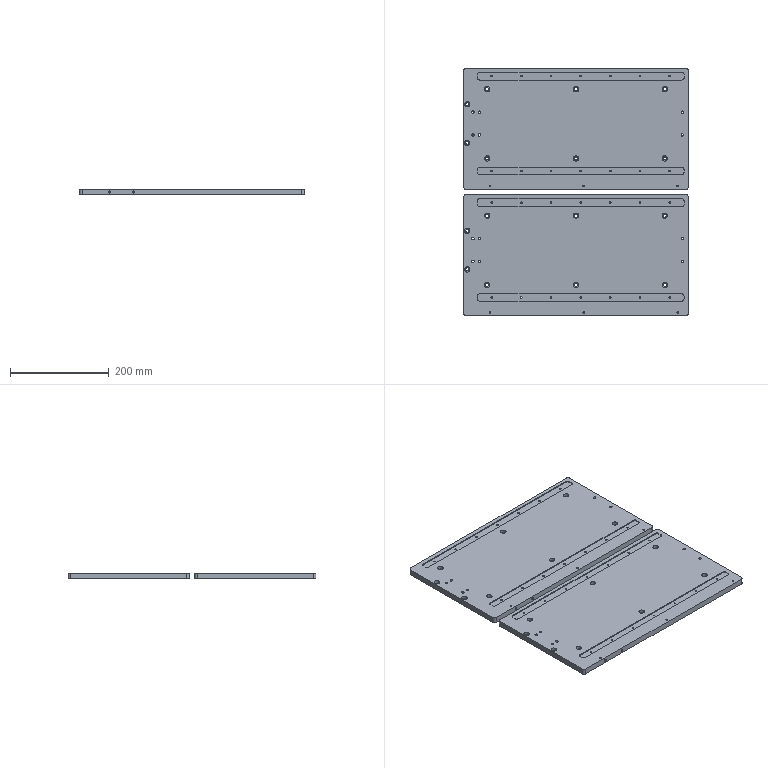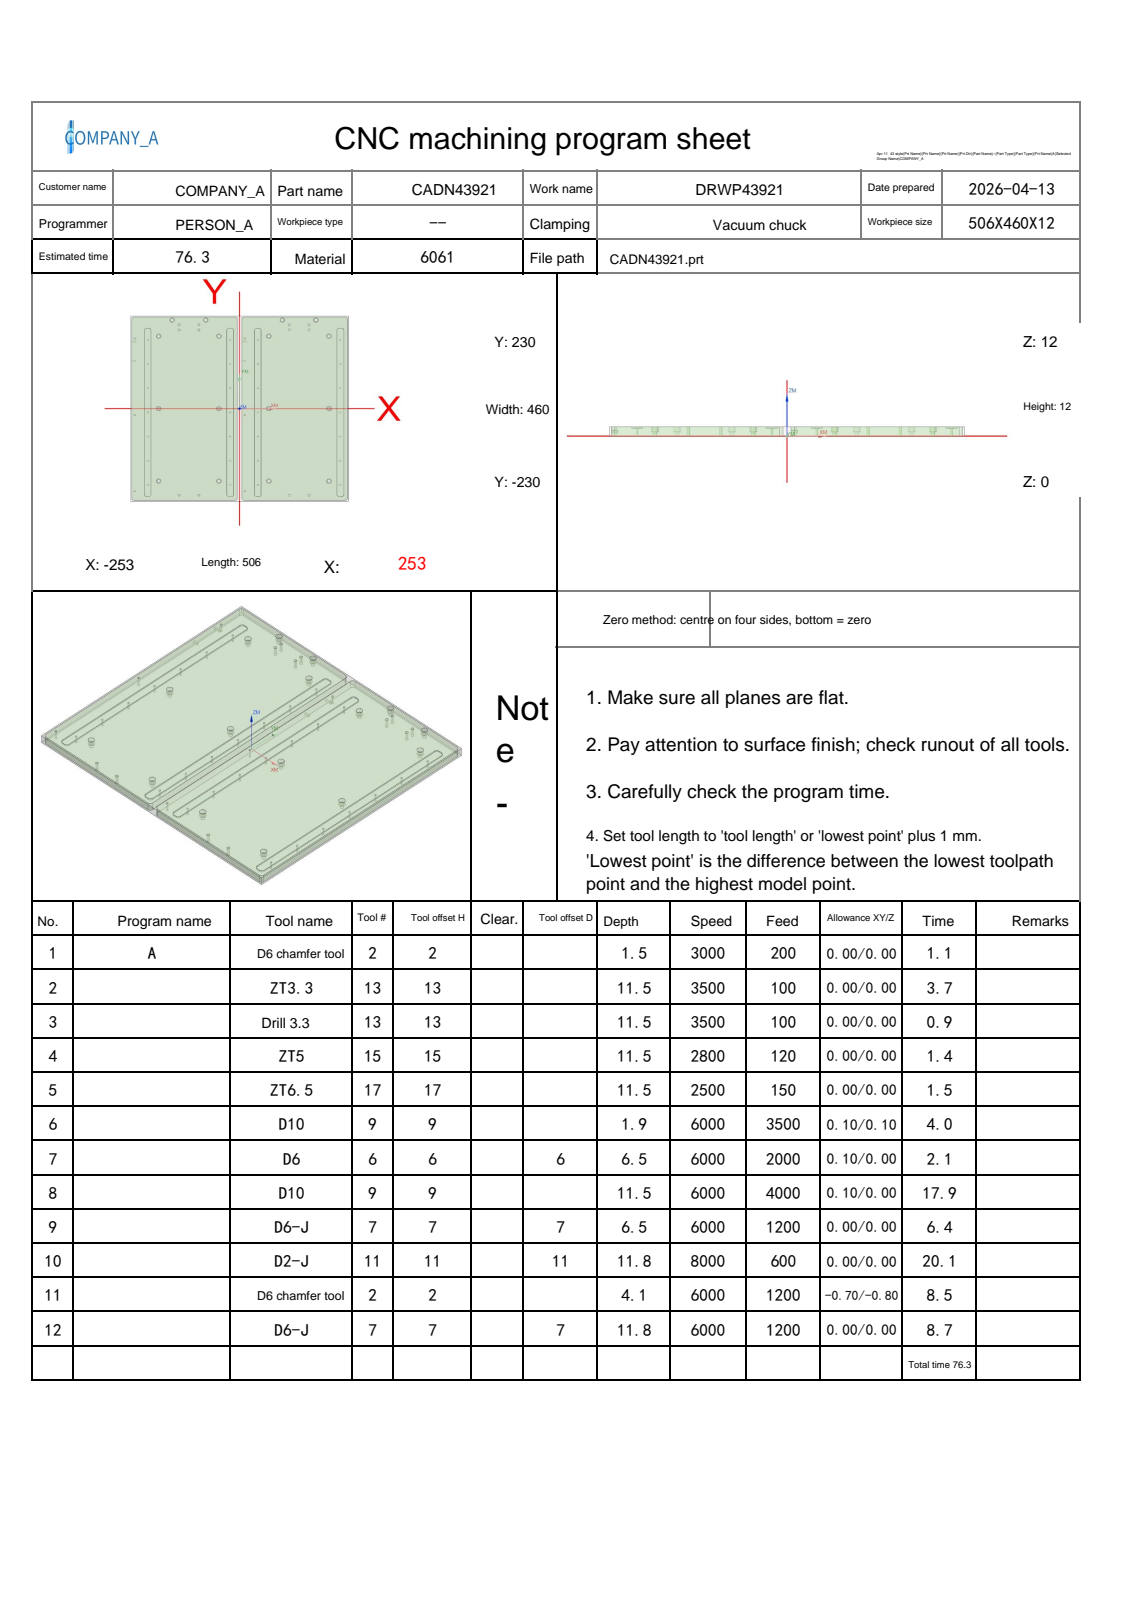NC program | NX | posted by the shop | part box 455 x 501 x 12 mm
Lines 10875 to 11580 of 11580:
N11 T02 M06
(D6 chamfer tool  D=6. R=0. H=02 ce=0.00 di=0.00)
G00 G90 G54 X3.672 Y-.25 M03 S6000
G43 H02 Z32.
M08
Z14.399
G01 Z10.501 F1200.
G03 X3.972 Y-.33 I.3 J.52
X4.492 Y-.03 I0.0 J.6
G01 X4.5 Y0.0
Y222.5
G02 X10.5 Y228.5 I6. J0.0
G01 X245.5
G02 X251.5 Y222.5 I0.0 J-6.
G01 Y-222.5
G02 X245.5 Y-228.5 I-6. J0.0
G01 X10.5
G02 X4.5 Y-222.5 I0.0 J6.
G01 Y0.0
X4.492 Y.03
G03 X3.972 Y.33 I-.52 J-.3
X3.672 Y.25 I0.0 J-.6
G01 Z14.399
G00 Z32.
X228.328 Y-9.25
Z14.399
G01 Z10.501
G03 X228.028 Y-9.17 I-.3 J-.52
X227.508 Y-9.47 I0.0 J-.6
G01 X227.5 Y-9.5
Y-213.5
G03 X231.7 Y-217.7 I4.2 J0.0
G01 X237.3
G03 X241.5 Y-213.5 I0.0 J4.2
G01 Y194.5
G03 X237.3 Y198.7 I-4.2 J0.0
G01 X231.7
G03 X227.5 Y194.5 I0.0 J-4.2
G01 Y-9.5
X227.508 Y-9.53
G03 X228.028 Y-9.83 I.52 J.3
X228.328 Y-9.75 I0.0 J.6
G01 Z14.399
G00 Z32.
X48.222
Z14.399
G01 Z10.501
G03 X48.522 Y-9.83 I.3 J.52
X49.042 Y-9.53 I0.0 J.6
G01 X49.05 Y-9.5
Y194.5
G03 X45. Y198.55 I-4.05 J0.0
G01 X40.
G03 X35.95 Y194.5 I0.0 J-4.05
G01 Y-213.5
G03 X40. Y-217.55 I4.05 J0.0
G01 X45.
G03 X49.05 Y-213.5 I0.0 J4.05
G01 Y-9.5
X49.042 Y-9.47
G03 X48.522 Y-9.17 I-.52 J-.3
X48.222 Y-9.25 I0.0 J-.6
G01 Z14.399
G00 Z32.
X-3.672 Y.25
Z14.399
G01 Z10.501
G03 X-3.972 Y.33 I-.3 J-.52
X-4.492 Y.03 I0.0 J-.6
G01 X-4.5 Y0.0
Y-222.5
G02 X-10.5 Y-228.5 I-6. J0.0
G01 X-245.5
G02 X-251.5 Y-222.5 I0.0 J6.
G01 Y222.5
G02 X-245.5 Y228.5 I6. J0.0
G01 X-10.5
G02 X-4.5 Y222.5 I0.0 J-6.
G01 Y0.0
X-4.492 Y-.03
G03 X-3.972 Y-.33 I.52 J.3
X-3.672 Y-.25 I0.0 J.6
G01 Z14.399
G00 Z32.
X-15.328 Y-9.75
Z14.399
G01 Z10.501
G03 X-15.028 Y-9.83 I.3 J.52
X-14.508 Y-9.53 I0.0 J.6
G01 X-14.5 Y-9.5
Y194.5
G03 X-18.7 Y198.7 I-4.2 J0.0
G01 X-24.3
G03 X-28.5 Y194.5 I0.0 J-4.2
G01 Y-213.5
G03 X-24.3 Y-217.7 I4.2 J0.0
G01 X-18.7
G03 X-14.5 Y-213.5 I0.0 J4.2
G01 Y-9.5
X-14.508 Y-9.47
G03 X-15.028 Y-9.17 I-.52 J-.3
X-15.328 Y-9.25 I0.0 J-.6
G01 Z14.399
G00 Z32.
X-207.778 Y-9.75
Z14.399
G01 Z10.501
G03 X-207.478 Y-9.83 I.3 J.52
X-206.958 Y-9.53 I0.0 J.6
G01 X-206.95 Y-9.5
Y194.5
G03 X-211. Y198.55 I-4.05 J0.0
G01 X-216.
G03 X-220.05 Y194.5 I0.0 J-4.05
G01 Y-213.5
G03 X-216. Y-217.55 I4.05 J0.0
G01 X-211.
G03 X-206.95 Y-213.5 I0.0 J4.05
G01 Y-9.5
X-206.958 Y-9.47
G03 X-207.478 Y-9.17 I-.52 J-.3
X-207.778 Y-9.25 I0.0 J-.6
G01 Z14.399
G00 Z32.
G00 G90 X-213.5 Y-189.5 M03 S5000
Z32.
G98 G81 X-213.5 Y-189.5 Z7.85 R13. F150.
Y-129.5
Y-69.5
Y-9.5
Y50.5
Y110.5
Y170.5
X-21.5 Y110.5
Y170.5
X42.5
Y110.5
Y50.5
X-21.5
Y-9.5
X42.5
Y-69.5
X-21.5
Y-129.5
Y-189.5
X42.5
Y-129.5
X234.5 Y-189.5
Y-129.5
Y-69.5
Y-9.5
Y50.5
Y110.5
Y170.5
G80
G00 Z32.
G00 G90 X-244. Y-205.678 M03 S5000
Z32.
G98 G81 X-244. Y-205.678 Z9.8 R15. F150.
Y-15.678
Y174.322
X12.
Y-15.678
Y-205.678
G80
G00 Z32.
G00 G90 X162.099 Y195.54 M03 S6000
Z32.
Z10.9
G01 Z10.4 F600.
X163. Y195.6
G03 X161.5 Y197.1 I-1.5 J0.0
X159.9 Y195.5 I0.0 J-1.6
X161.5 Y193.9 I1.6 J0.0
X163.1 Y195.5 I0.0 J1.6
X161.5 Y197.1 I-1.6 J0.0
X160. Y195.6 I0.0 J-1.5
G01 X160.901 Y195.54
Z10.9
G00 Z32.
X162.099 Y208.54
Z10.9
G01 Z10.4
X163. Y208.6
G03 X161.5 Y210.1 I-1.5 J0.0
X159.9 Y208.5 I0.0 J-1.6
X161.5 Y206.9 I1.6 J0.0
X163.1 Y208.5 I0.0 J1.6
X161.5 Y210.1 I-1.6 J0.0
X160. Y208.6 I0.0 J-1.5
G01 X160.901 Y208.54
Z10.9
G00 Z32.
X116.099
Z10.9
G01 Z10.4
X117. Y208.6
G03 X115.5 Y210.1 I-1.5 J0.0
X113.9 Y208.5 I0.0 J-1.6
X115.5 Y206.9 I1.6 J0.0
X117.1 Y208.5 I0.0 J1.6
X115.5 Y210.1 I-1.6 J0.0
X114. Y208.6 I0.0 J-1.5
G01 X114.901 Y208.54
Z10.9
G00 Z32.
X116.099 Y195.54
Z10.9
G01 Z10.4
X117. Y195.6
G03 X115.5 Y197.1 I-1.5 J0.0
X113.9 Y195.5 I0.0 J-1.6
X115.5 Y193.9 I1.6 J0.0
X117.1 Y195.5 I0.0 J1.6
X115.5 Y197.1 I-1.6 J0.0
X114. Y195.6 I0.0 J-1.5
G01 X114.901 Y195.54
Z10.9
G00 Z32.
X-93.901
Z10.9
G01 Z10.4
X-93. Y195.6
G03 X-94.5 Y197.1 I-1.5 J0.0
X-96.1 Y195.5 I0.0 J-1.6
X-94.5 Y193.9 I1.6 J0.0
X-92.9 Y195.5 I0.0 J1.6
X-94.5 Y197.1 I-1.6 J0.0
X-96. Y195.6 I0.0 J-1.5
G01 X-95.099 Y195.54
Z10.9
G00 Z32.
X-93.901 Y208.54
Z10.9
G01 Z10.4
X-93. Y208.6
G03 X-94.5 Y210.1 I-1.5 J0.0
X-96.1 Y208.5 I0.0 J-1.6
X-94.5 Y206.9 I1.6 J0.0
X-92.9 Y208.5 I0.0 J1.6
X-94.5 Y210.1 I-1.6 J0.0
X-96. Y208.6 I0.0 J-1.5
G01 X-95.099 Y208.54
Z10.9
G00 Z32.
X-139.901
Z10.9
G01 Z10.4
X-139. Y208.6
G03 X-140.5 Y210.1 I-1.5 J0.0
X-142.1 Y208.5 I0.0 J-1.6
X-140.5 Y206.9 I1.6 J0.0
X-138.9 Y208.5 I0.0 J1.6
X-140.5 Y210.1 I-1.6 J0.0
X-142. Y208.6 I0.0 J-1.5
G01 X-141.099 Y208.54
Z10.9
G00 Z32.
X-139.901 Y195.54
Z10.9
G01 Z10.4
X-139. Y195.6
G03 X-140.5 Y197.1 I-1.5 J0.0
X-142.1 Y195.5 I0.0 J-1.6
X-140.5 Y193.9 I1.6 J0.0
X-138.9 Y195.5 I0.0 J1.6
X-140.5 Y197.1 I-1.6 J0.0
X-142. Y195.6 I0.0 J-1.5
G01 X-141.099 Y195.54
Z10.9
G00 Z32.
X-139.901 Y-214.96
Z10.9
G01 Z10.4
X-139. Y-214.9
G03 X-140.5 Y-213.4 I-1.5 J0.0
X-142.1 Y-215. I0.0 J-1.6
X-140.5 Y-216.6 I1.6 J0.0
X-138.9 Y-215. I0.0 J1.6
X-140.5 Y-213.4 I-1.6 J0.0
X-142. Y-214.9 I0.0 J-1.5
G01 X-141.099 Y-214.96
Z10.9
G00 Z32.
X-93.901
Z10.9
G01 Z10.4
X-93. Y-214.9
G03 X-94.5 Y-213.4 I-1.5 J0.0
X-96.1 Y-215. I0.0 J-1.6
X-94.5 Y-216.6 I1.6 J0.0
X-92.9 Y-215. I0.0 J1.6
X-94.5 Y-213.4 I-1.6 J0.0
X-96. Y-214.9 I0.0 J-1.5
G01 X-95.099 Y-214.96
Z10.9
G00 Z32.
X116.099
Z10.9
G01 Z10.4
X117. Y-214.9
G03 X115.5 Y-213.4 I-1.5 J0.0
X113.9 Y-215. I0.0 J-1.6
X115.5 Y-216.6 I1.6 J0.0
X117.1 Y-215. I0.0 J1.6
X115.5 Y-213.4 I-1.6 J0.0
X114. Y-214.9 I0.0 J-1.5
G01 X114.901 Y-214.96
Z10.9
G00 Z32.
X162.099
Z10.9
G01 Z10.4
X163. Y-214.9
G03 X161.5 Y-213.4 I-1.5 J0.0
X159.9 Y-215. I0.0 J-1.6
X161.5 Y-216.6 I1.6 J0.0
X163.1 Y-215. I0.0 J1.6
X161.5 Y-213.4 I-1.6 J0.0
X160. Y-214.9 I0.0 J-1.5
G01 X160.901 Y-214.96
Z10.9
G00 Z32.
G00 G90 X211. Y180.001 M03 S6000
Z32.
Z10.5
G01 Z10. F600.
Y181.
G03 X208. Y184. I-3. J0.0
X204. Y180. I0.0 J-4.
X208. Y176. I4. J0.0
X212. Y180. I0.0 J4.
X208. Y184. I-4. J0.0
X205. Y181. I0.0 J-3.
G01 Y180.001
Z10.5
G00 Z32.
X180.5 Y220.001
Z10.5
G01 Z10.
Y221.
G03 X177.5 Y224. I-3. J0.0
X173.5 Y220. I0.0 J-4.
X177.5 Y216. I4. J0.0
X181.5 Y220. I0.0 J4.
X177.5 Y224. I-4. J0.0
X174.5 Y221. I0.0 J-3.
G01 Y220.001
Z10.5
G00 Z32.
X102.5
Z10.5
G01 Z10.
Y221.
G03 X99.5 Y224. I-3. J0.0
X95.5 Y220. I0.0 J-4.
X99.5 Y216. I4. J0.0
X103.5 Y220. I0.0 J4.
X99.5 Y224. I-4. J0.0
X96.5 Y221. I0.0 J-3.
G01 Y220.001
Z10.5
G00 Z32.
X71. Y180.001
Z10.5
G01 Z10.
Y181.
G03 X68. Y184. I-3. J0.0
X64. Y180. I0.0 J-4.
X68. Y176. I4. J0.0
X72. Y180. I0.0 J4.
X68. Y184. I-4. J0.0
X65. Y181. I0.0 J-3.
G01 Y180.001
Z10.5
G00 Z32.
X-45.
Z10.5
G01 Z10.
Y181.
G03 X-48. Y184. I-3. J0.0
X-52. Y180. I0.0 J-4.
X-48. Y176. I4. J0.0
X-44. Y180. I0.0 J4.
X-48. Y184. I-4. J0.0
X-51. Y181. I0.0 J-3.
G01 Y180.001
Z10.5
G00 Z32.
X-75.5 Y220.001
Z10.5
G01 Z10.
Y221.
G03 X-78.5 Y224. I-3. J0.0
X-82.5 Y220. I0.0 J-4.
X-78.5 Y216. I4. J0.0
X-74.5 Y220. I0.0 J4.
X-78.5 Y224. I-4. J0.0
X-81.5 Y221. I0.0 J-3.
G01 Y220.001
Z10.5
G00 Z32.
X-153.5
Z10.5
G01 Z10.
Y221.
G03 X-156.5 Y224. I-3. J0.0
X-160.5 Y220. I0.0 J-4.
X-156.5 Y216. I4. J0.0
X-152.5 Y220. I0.0 J4.
X-156.5 Y224. I-4. J0.0
X-159.5 Y221. I0.0 J-3.
G01 Y220.001
Z10.5
G00 Z32.
X-185. Y180.001
Z10.5
G01 Z10.
Y181.
G03 X-188. Y184. I-3. J0.0
X-192. Y180. I0.0 J-4.
X-188. Y176. I4. J0.0
X-184. Y180. I0.0 J4.
X-188. Y184. I-4. J0.0
X-191. Y181. I0.0 J-3.
G01 Y180.001
Z10.5
G00 Z32.
X-185. Y.001
Z10.5
G01 Z10.
Y1.
G03 X-188. Y4. I-3. J0.0
X-192. Y0.0 I0.0 J-4.
X-188. Y-4. I4. J0.0
X-184. Y0.0 I0.0 J4.
X-188. Y4. I-4. J0.0
X-191. Y1. I0.0 J-3.
G01 Y.001
Z10.5
G00 Z32.
X-45.
Z10.5
G01 Z10.
Y1.
G03 X-48. Y4. I-3. J0.0
X-52. Y0.0 I0.0 J-4.
X-48. Y-4. I4. J0.0
X-44. Y0.0 I0.0 J4.
X-48. Y4. I-4. J0.0
X-51. Y1. I0.0 J-3.
G01 Y.001
Z10.5
G00 Z32.
X71.
Z10.5
G01 Z10.
Y1.
G03 X68. Y4. I-3. J0.0
X64. Y0.0 I0.0 J-4.
X68. Y-4. I4. J0.0
X72. Y0.0 I0.0 J4.
X68. Y4. I-4. J0.0
X65. Y1. I0.0 J-3.
G01 Y.001
Z10.5
G00 Z32.
X211.
Z10.5
G01 Z10.
Y1.
G03 X208. Y4. I-3. J0.0
X204. Y0.0 I0.0 J-4.
X208. Y-4. I4. J0.0
X212. Y0.0 I0.0 J4.
X208. Y4. I-4. J0.0
X205. Y1. I0.0 J-3.
G01 Y.001
Z10.5
G00 Z32.
X211. Y-179.999
Z10.5
G01 Z10.
Y-179.
G03 X208. Y-176. I-3. J0.0
X204. Y-180. I0.0 J-4.
X208. Y-184. I4. J0.0
X212. Y-180. I0.0 J4.
X208. Y-176. I-4. J0.0
X205. Y-179. I0.0 J-3.
G01 Y-179.999
Z10.5
G00 Z32.
X71.
Z10.5
G01 Z10.
Y-179.
G03 X68. Y-176. I-3. J0.0
X64. Y-180. I0.0 J-4.
X68. Y-184. I4. J0.0
X72. Y-180. I0.0 J4.
X68. Y-176. I-4. J0.0
X65. Y-179. I0.0 J-3.
G01 Y-179.999
Z10.5
G00 Z32.
X-45.
Z10.5
G01 Z10.
Y-179.
G03 X-48. Y-176. I-3. J0.0
X-52. Y-180. I0.0 J-4.
X-48. Y-184. I4. J0.0
X-44. Y-180. I0.0 J4.
X-48. Y-176. I-4. J0.0
X-51. Y-179. I0.0 J-3.
G01 Y-179.999
Z10.5
G00 Z32.
X-185.
Z10.5
G01 Z10.
Y-179.
G03 X-188. Y-176. I-3. J0.0
X-192. Y-180. I0.0 J-4.
X-188. Y-184. I4. J0.0
X-184. Y-180. I0.0 J4.
X-188. Y-176. I-4. J0.0
X-191. Y-179. I0.0 J-3.
G01 Y-179.999
Z10.5
G00 Z32.
G91 G28 Z0.0
M05
M09
G91 G28 Z0.0
M01
N12 T07 M06
(D6-J  D=6. R=0. H=07 ce=0.00 di=0.01)
G00 G90 G54 X238.4 Y-10.5 M03 S6000
G43 H07 Z32.
M08
Z10.505
G01 Z10.005 F1200.
G41 D07
X238.5
G03 X239.5 Y-9.5 I0.0 J1.
G01 Y194.5
G03 X237.3 Y196.7 I-2.2 J0.0
G01 X231.7
G03 X229.5 Y194.5 I0.0 J-2.2
G01 Y-213.5
G03 X231.7 Y-215.7 I2.2 J0.0
G01 X237.3
G03 X239.5 Y-213.5 I0.0 J2.2
G01 Y-9.5
Y-9.
G03 X238.5 Y-8. I-1. J0.0
G01 G40 X238.4
Z10.505
G00 Z32.
X-17.6 Y-10.5
Z10.505
G01 Z10.005
G41 D07
X-17.5
G03 X-16.5 Y-9.5 I0.0 J1.
G01 Y194.5
G03 X-18.7 Y196.7 I-2.2 J0.0
G01 X-24.3
G03 X-26.5 Y194.5 I0.0 J-2.2
G01 Y-213.5
G03 X-24.3 Y-215.7 I2.2 J0.0
G01 X-18.7
G03 X-16.5 Y-213.5 I0.0 J2.2
G01 Y-9.5
Y-9.
G03 X-17.5 Y-8. I-1. J0.0
G01 G40 X-17.6
Z10.505
G00 Z32.
G00 G90 X45.95 Y-10.5 M03 S6000
Z32.
Z10.505
G01 Z10.005 F1200.
G41 D07
X46.05
G03 X47.05 Y-9.5 I0.0 J1.
G01 Y194.5
G03 X45. Y196.55 I-2.05 J0.0
G01 X40.
G03 X37.95 Y194.5 I0.0 J-2.05
G01 Y-213.5
G03 X40. Y-215.55 I2.05 J0.0
G01 X45.
G03 X47.05 Y-213.5 I0.0 J2.05
G01 Y-9.5
Y-9.
G03 X46.05 Y-8. I-1. J0.0
G01 G40 X45.95
Z10.505
G00 Z32.
X-216.95 Y-8.5
Z10.505
G01 Z10.005
G41 D07
X-217.05
G03 X-218.05 Y-9.5 I0.0 J-1.
G01 Y-213.5
G03 X-216. Y-215.55 I2.05 J0.0
G01 X-211.
G03 X-208.95 Y-213.5 I0.0 J2.05
G01 Y194.5
G03 X-211. Y196.55 I-2.05 J0.0
G01 X-216.
G03 X-218.05 Y194.5 I0.0 J-2.05
G01 Y-9.5
Y-10.
G03 X-217.05 Y-11. I1. J0.0
G01 G40 X-216.95
Z10.505
G00 Z32.
G00 G90 X-254.644 Y-223.51 M03 S6000
Z32.
Z1.
G01 Z.5 F1000.
G41 D07
X-254.444 Y-223.498
G03 X-253.5 Y-222.5 I-.056 J.998
G01 Y222.5
G02 X-245.5 Y230.5 I8. J0.0
G01 X-10.5
G02 X-2.5 Y222.5 I0.0 J-8.
G01 Y-222.5
G02 X-10.5 Y-230.5 I-8. J0.0
G01 X-245.5
G02 X-253.5 Y-222.5 I0.0 J8.
G01 Y-222.
G03 X-254.5 Y-221. I-1. J0.0
G01 G40 X-254.7
Z1.
G00 Z32.
X254.644 Y223.51
Z1.
G01 Z.5
G41 D07
X254.444 Y223.498
G03 X253.5 Y222.5 I.056 J-.998
G01 Y-222.5
G02 X245.5 Y-230.5 I-8. J0.0
G01 X10.5
G02 X2.5 Y-222.5 I0.0 J8.
G01 Y222.5
G02 X10.5 Y230.5 I8. J0.0
G01 X245.5
G02 X253.5 Y222.5 I0.0 J-8.
G01 Y222.
G03 X254.5 Y221. I1. J0.0
G01 G40 X254.7
Z1.
G00 Z32.
G00 G90 X-254.544 Y-223.504 M03 S6000
Z32.
Z.7
G01 Z.2 F1000.
G41 D07
X-254.444 Y-223.498
G03 X-253.5 Y-222.5 I-.056 J.998
G01 Y222.5
G02 X-245.5 Y230.5 I8. J0.0
G01 X-10.5
G02 X-2.5 Y222.5 I0.0 J-8.
G01 Y-222.5
G02 X-10.5 Y-230.5 I-8. J0.0
G01 X-245.5
G02 X-253.5 Y-222.5 I0.0 J8.
G01 Y-222.
G03 X-254.5 Y-221. I-1. J0.0
G01 G40 X-254.6
Z.7
G00 Z32.
X254.544 Y223.504
Z.7
G01 Z.2
G41 D07
X254.444 Y223.498
G03 X253.5 Y222.5 I.056 J-.998
G01 Y-222.5
G02 X245.5 Y-230.5 I-8. J0.0
G01 X10.5
G02 X2.5 Y-222.5 I0.0 J8.
G01 Y222.5
G02 X10.5 Y230.5 I8. J0.0
G01 X245.5
G02 X253.5 Y222.5 I0.0 J-8.
G01 Y222.
G03 X254.5 Y221. I1. J0.0
G01 G40 X254.6
Z.7
G00 Z32.
M05
M09
G91 G28 Z0.0
G91 G28 Y0.0
M30
%